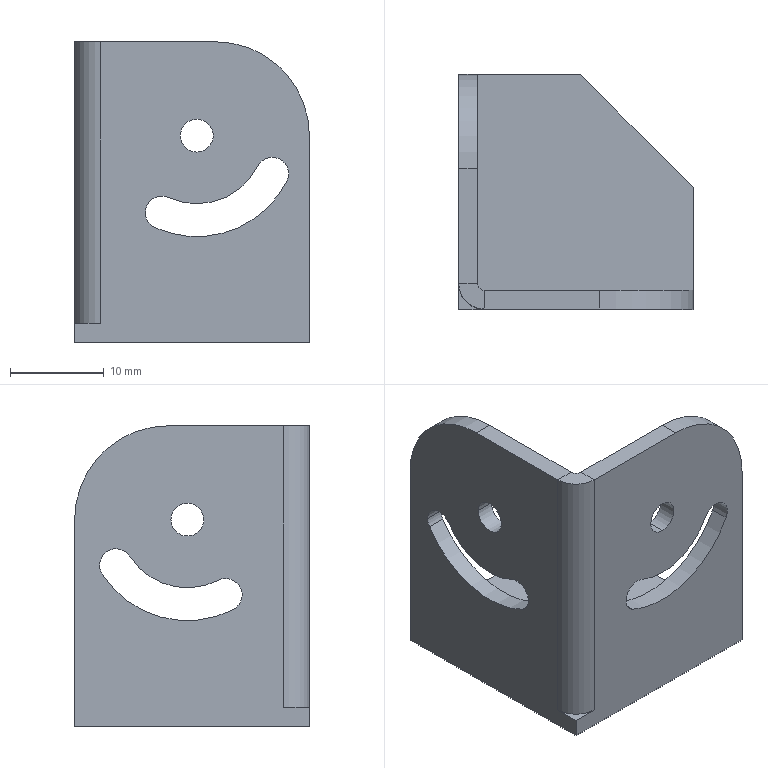Part | STEP file | 11-TG-00211 | 1 solid | 32 faces | box 25 x 25 x 32 mm | volume 3589 mm3 | cylinder 19 | plane 13 | commonest cylinder face diameters 3.5 x11 14.5 x2 20 x2 21.5 x2 1.473 x1 5.473 x1
STEP:
#1=CARTESIAN_POINT('',(19.033,-2.,17.692));
#2=VERTEX_POINT('',#1);
#3=CARTESIAN_POINT('',(20.595,-2.,15.153));
#4=VERTEX_POINT('',#3);
#5=CARTESIAN_POINT('',(19.033,-2.,15.942));
#6=DIRECTION('',(0.,1.,0.));
#7=DIRECTION('',(0.,0.,1.));
#8=AXIS2_PLACEMENT_3D('',#5,#6,#7);
#9=CIRCLE('',#8,1.75);
#10=EDGE_CURVE('',#2,#4,#9,.T.);
#11=ORIENTED_EDGE('',*,*,#10,.F.);
#12=CARTESIAN_POINT('',(19.033,0.,17.692));
#13=VERTEX_POINT('',#12);
#14=CARTESIAN_POINT('',(19.033,-10.,17.692));
#15=DIRECTION('',(0.,1.,0.));
#16=VECTOR('',#15,1000.);
#17=LINE('',#14,#16);
#18=EDGE_CURVE('',#2,#13,#17,.T.);
#19=ORIENTED_EDGE('',*,*,#18,.T.);
#20=CARTESIAN_POINT('',(20.595,0.,15.153));
#21=VERTEX_POINT('',#20);
#22=CARTESIAN_POINT('',(19.033,0.,15.942));
#23=DIRECTION('',(0.,1.,0.));
#24=DIRECTION('',(0.,0.,1.));
#25=AXIS2_PLACEMENT_3D('',#22,#23,#24);
#26=CIRCLE('',#25,1.75);
#27=EDGE_CURVE('',#13,#21,#26,.T.);
#28=ORIENTED_EDGE('',*,*,#27,.T.);
#29=CARTESIAN_POINT('',(20.595,-10.,15.153));
#30=DIRECTION('',(0.,1.,0.));
#31=VECTOR('',#30,1000.);
#32=LINE('',#29,#31);
#33=EDGE_CURVE('',#4,#21,#32,.T.);
#34=ORIENTED_EDGE('',*,*,#33,.F.);
#35=EDGE_LOOP('',(#11,#19,#28,#34));
#36=FACE_OUTER_BOUND('',#35,.T.);
#37=CARTESIAN_POINT('',(19.033,-10.,15.942));
#38=DIRECTION('',(0.,1.,0.));
#39=DIRECTION('',(0.,0.,1.));
#40=AXIS2_PLACEMENT_3D('',#37,#38,#39);
#41=CYLINDRICAL_SURFACE('',#40,1.75);
#42=ADVANCED_FACE('',(#36),#41,.F.);
#43=CARTESIAN_POINT('',(7.279,-2.,13.555));
#44=VERTEX_POINT('',#43);
#45=CARTESIAN_POINT('',(8.002,-2.,13.399));
#46=VERTEX_POINT('',#45);
#47=CARTESIAN_POINT('',(7.279,-2.,11.805));
#48=DIRECTION('',(0.,1.,0.));
#49=DIRECTION('',(0.,0.,1.));
#50=AXIS2_PLACEMENT_3D('',#47,#48,#49);
#51=CIRCLE('',#50,1.75);
#52=EDGE_CURVE('',#44,#46,#51,.T.);
#53=ORIENTED_EDGE('',*,*,#52,.F.);
#54=CARTESIAN_POINT('',(7.279,0.,13.555));
#55=VERTEX_POINT('',#54);
#56=CARTESIAN_POINT('',(7.279,-10.,13.555));
#57=DIRECTION('',(0.,1.,0.));
#58=VECTOR('',#57,1000.);
#59=LINE('',#56,#58);
#60=EDGE_CURVE('',#44,#55,#59,.T.);
#61=ORIENTED_EDGE('',*,*,#60,.T.);
#62=CARTESIAN_POINT('',(8.002,0.,13.399));
#63=VERTEX_POINT('',#62);
#64=CARTESIAN_POINT('',(7.279,0.,11.805));
#65=DIRECTION('',(0.,1.,0.));
#66=DIRECTION('',(0.,0.,1.));
#67=AXIS2_PLACEMENT_3D('',#64,#65,#66);
#68=CIRCLE('',#67,1.75);
#69=EDGE_CURVE('',#55,#63,#68,.T.);
#70=ORIENTED_EDGE('',*,*,#69,.T.);
#71=CARTESIAN_POINT('',(8.002,-10.,13.399));
#72=DIRECTION('',(0.,1.,0.));
#73=VECTOR('',#72,1000.);
#74=LINE('',#71,#73);
#75=EDGE_CURVE('',#46,#63,#74,.T.);
#76=ORIENTED_EDGE('',*,*,#75,.F.);
#77=EDGE_LOOP('',(#53,#61,#70,#76));
#78=FACE_OUTER_BOUND('',#77,.T.);
#79=CARTESIAN_POINT('',(7.279,-10.,11.805));
#80=DIRECTION('',(0.,1.,0.));
#81=DIRECTION('',(0.,0.,1.));
#82=AXIS2_PLACEMENT_3D('',#79,#80,#81);
#83=CYLINDRICAL_SURFACE('',#82,1.75);
#84=ADVANCED_FACE('',(#78),#83,.F.);
#85=CARTESIAN_POINT('',(11.,-2.,18.25));
#86=VERTEX_POINT('',#85);
#87=CARTESIAN_POINT('',(11.,-2.,21.75));
#88=VERTEX_POINT('',#87);
#89=CARTESIAN_POINT('',(11.,-2.,20.));
#90=DIRECTION('',(0.,1.,0.));
#91=DIRECTION('',(0.,0.,1.));
#92=AXIS2_PLACEMENT_3D('',#89,#90,#91);
#93=CIRCLE('',#92,1.75);
#94=EDGE_CURVE('',#86,#88,#93,.T.);
#95=ORIENTED_EDGE('',*,*,#94,.F.);
#96=CARTESIAN_POINT('',(11.,0.,18.25));
#97=VERTEX_POINT('',#96);
#98=CARTESIAN_POINT('',(11.,-10.,18.25));
#99=DIRECTION('',(0.,1.,0.));
#100=VECTOR('',#99,1000.);
#101=LINE('',#98,#100);
#102=EDGE_CURVE('',#86,#97,#101,.T.);
#103=ORIENTED_EDGE('',*,*,#102,.T.);
#104=CARTESIAN_POINT('',(11.,0.,21.75));
#105=VERTEX_POINT('',#104);
#106=CARTESIAN_POINT('',(11.,0.,20.));
#107=DIRECTION('',(0.,1.,0.));
#108=DIRECTION('',(0.,0.,1.));
#109=AXIS2_PLACEMENT_3D('',#106,#107,#108);
#110=CIRCLE('',#109,1.75);
#111=EDGE_CURVE('',#97,#105,#110,.T.);
#112=ORIENTED_EDGE('',*,*,#111,.T.);
#113=CARTESIAN_POINT('',(11.,-10.,21.75));
#114=DIRECTION('',(0.,1.,0.));
#115=VECTOR('',#114,1000.);
#116=LINE('',#113,#115);
#117=EDGE_CURVE('',#88,#105,#116,.T.);
#118=ORIENTED_EDGE('',*,*,#117,.F.);
#119=EDGE_LOOP('',(#95,#103,#112,#118));
#120=FACE_OUTER_BOUND('',#119,.T.);
#121=CARTESIAN_POINT('',(11.,-10.,20.));
#122=DIRECTION('',(0.,1.,0.));
#123=DIRECTION('',(0.,0.,1.));
#124=AXIS2_PLACEMENT_3D('',#121,#122,#123);
#125=CYLINDRICAL_SURFACE('',#124,1.75);
#126=ADVANCED_FACE('',(#120),#125,.F.);
#127=CARTESIAN_POINT('',(-2.,20.331,15.15));
#128=VERTEX_POINT('',#127);
#129=CARTESIAN_POINT('',(-2.,17.107,16.093));
#130=VERTEX_POINT('',#129);
#131=CARTESIAN_POINT('',(-2.,18.581,15.15));
#132=DIRECTION('',(1.,0.,0.));
#133=DIRECTION('',(0.,1.,0.));
#134=AXIS2_PLACEMENT_3D('',#131,#132,#133);
#135=CIRCLE('',#134,1.75);
#136=EDGE_CURVE('',#128,#130,#135,.T.);
#137=ORIENTED_EDGE('',*,*,#136,.F.);
#138=CARTESIAN_POINT('',(0.,20.331,15.15));
#139=VERTEX_POINT('',#138);
#140=CARTESIAN_POINT('',(-10.,20.331,15.15));
#141=DIRECTION('',(1.,0.,0.));
#142=VECTOR('',#141,1000.);
#143=LINE('',#140,#142);
#144=EDGE_CURVE('',#128,#139,#143,.T.);
#145=ORIENTED_EDGE('',*,*,#144,.T.);
#146=CARTESIAN_POINT('',(0.,17.107,16.093));
#147=VERTEX_POINT('',#146);
#148=CARTESIAN_POINT('',(0.,18.581,15.15));
#149=DIRECTION('',(1.,0.,0.));
#150=DIRECTION('',(0.,1.,0.));
#151=AXIS2_PLACEMENT_3D('',#148,#149,#150);
#152=CIRCLE('',#151,1.75);
#153=EDGE_CURVE('',#139,#147,#152,.T.);
#154=ORIENTED_EDGE('',*,*,#153,.T.);
#155=CARTESIAN_POINT('',(-10.,17.107,16.093));
#156=DIRECTION('',(1.,0.,0.));
#157=VECTOR('',#156,1000.);
#158=LINE('',#155,#157);
#159=EDGE_CURVE('',#130,#147,#158,.T.);
#160=ORIENTED_EDGE('',*,*,#159,.F.);
#161=EDGE_LOOP('',(#137,#145,#154,#160));
#162=FACE_OUTER_BOUND('',#161,.T.);
#163=CARTESIAN_POINT('',(-10.,18.581,15.15));
#164=DIRECTION('',(1.,0.,0.));
#165=DIRECTION('',(0.,1.,0.));
#166=AXIS2_PLACEMENT_3D('',#163,#164,#165);
#167=CYLINDRICAL_SURFACE('',#166,1.75);
#168=ADVANCED_FACE('',(#162),#167,.F.);
#169=CARTESIAN_POINT('',(-2.,9.25,20.));
#170=VERTEX_POINT('',#169);
#171=CARTESIAN_POINT('',(-2.,12.75,20.));
#172=VERTEX_POINT('',#171);
#173=CARTESIAN_POINT('',(-2.,11.,20.));
#174=DIRECTION('',(1.,0.,0.));
#175=DIRECTION('',(0.,1.,0.));
#176=AXIS2_PLACEMENT_3D('',#173,#174,#175);
#177=CIRCLE('',#176,1.75);
#178=EDGE_CURVE('',#170,#172,#177,.T.);
#179=ORIENTED_EDGE('',*,*,#178,.F.);
#180=CARTESIAN_POINT('',(0.,9.25,20.));
#181=VERTEX_POINT('',#180);
#182=CARTESIAN_POINT('',(-10.,9.25,20.));
#183=DIRECTION('',(1.,0.,0.));
#184=VECTOR('',#183,1000.);
#185=LINE('',#182,#184);
#186=EDGE_CURVE('',#170,#181,#185,.T.);
#187=ORIENTED_EDGE('',*,*,#186,.T.);
#188=CARTESIAN_POINT('',(0.,12.75,20.));
#189=VERTEX_POINT('',#188);
#190=CARTESIAN_POINT('',(0.,11.,20.));
#191=DIRECTION('',(1.,0.,0.));
#192=DIRECTION('',(0.,1.,0.));
#193=AXIS2_PLACEMENT_3D('',#190,#191,#192);
#194=CIRCLE('',#193,1.75);
#195=EDGE_CURVE('',#181,#189,#194,.T.);
#196=ORIENTED_EDGE('',*,*,#195,.T.);
#197=CARTESIAN_POINT('',(-10.,12.75,20.));
#198=DIRECTION('',(1.,0.,0.));
#199=VECTOR('',#198,1000.);
#200=LINE('',#197,#199);
#201=EDGE_CURVE('',#172,#189,#200,.T.);
#202=ORIENTED_EDGE('',*,*,#201,.F.);
#203=EDGE_LOOP('',(#179,#187,#196,#202));
#204=FACE_OUTER_BOUND('',#203,.T.);
#205=CARTESIAN_POINT('',(-10.,11.,20.));
#206=DIRECTION('',(1.,0.,0.));
#207=DIRECTION('',(0.,1.,0.));
#208=AXIS2_PLACEMENT_3D('',#205,#206,#207);
#209=CYLINDRICAL_SURFACE('',#208,1.75);
#210=ADVANCED_FACE('',(#204),#209,.F.);
#211=CARTESIAN_POINT('',(11.,-2.,20.));
#212=DIRECTION('',(0.,1.,0.));
#213=DIRECTION('',(0.,0.,1.));
#214=AXIS2_PLACEMENT_3D('',#211,#212,#213);
#215=CIRCLE('',#214,1.75);
#216=EDGE_CURVE('',#88,#86,#215,.T.);
#217=ORIENTED_EDGE('',*,*,#216,.T.);
#218=ORIENTED_EDGE('',*,*,#94,.T.);
#219=EDGE_LOOP('',(#217,#218));
#220=FACE_BOUND('',#219,.T.);
#221=CARTESIAN_POINT('',(23.,-2.,20.));
#222=VERTEX_POINT('',#221);
#223=CARTESIAN_POINT('',(23.,-2.,-2.));
#224=VERTEX_POINT('',#223);
#225=CARTESIAN_POINT('',(23.,-2.,30.));
#226=DIRECTION('',(0.,0.,-1.));
#227=VECTOR('',#226,1000.);
#228=LINE('',#225,#227);
#229=EDGE_CURVE('',#222,#224,#228,.T.);
#230=ORIENTED_EDGE('',*,*,#229,.F.);
#231=CARTESIAN_POINT('',(13.,-2.,30.));
#232=VERTEX_POINT('',#231);
#233=CARTESIAN_POINT('',(13.,-2.,20.));
#234=DIRECTION('',(0.,-1.,0.));
#235=DIRECTION('',(0.,0.,1.));
#236=AXIS2_PLACEMENT_3D('',#233,#234,#235);
#237=CIRCLE('',#236,10.);
#238=EDGE_CURVE('',#222,#232,#237,.T.);
#239=ORIENTED_EDGE('',*,*,#238,.T.);
#240=CARTESIAN_POINT('',(0.7366,-2.,30.));
#241=VERTEX_POINT('',#240);
#242=CARTESIAN_POINT('',(0.,-2.,30.));
#243=DIRECTION('',(1.,0.,0.));
#244=VECTOR('',#243,1000.);
#245=LINE('',#242,#244);
#246=EDGE_CURVE('',#241,#232,#245,.T.);
#247=ORIENTED_EDGE('',*,*,#246,.F.);
#248=CARTESIAN_POINT('',(0.7366,-2.,0.));
#249=VERTEX_POINT('',#248);
#250=CARTESIAN_POINT('',(0.7366,-2.,30.));
#251=DIRECTION('',(0.,0.,-1.));
#252=VECTOR('',#251,1000.);
#253=LINE('',#250,#252);
#254=EDGE_CURVE('',#241,#249,#253,.T.);
#255=ORIENTED_EDGE('',*,*,#254,.T.);
#256=CARTESIAN_POINT('',(-2.,-2.,0.));
#257=VERTEX_POINT('',#256);
#258=CARTESIAN_POINT('',(23.,-2.,0.));
#259=DIRECTION('',(-1.,0.,0.));
#260=VECTOR('',#259,1000.);
#261=LINE('',#258,#260);
#262=EDGE_CURVE('',#249,#257,#261,.T.);
#263=ORIENTED_EDGE('',*,*,#262,.T.);
#264=CARTESIAN_POINT('',(-2.,-2.,-2.));
#265=VERTEX_POINT('',#264);
#266=CARTESIAN_POINT('',(-2.,-2.,-2.));
#267=DIRECTION('',(0.,0.,1.));
#268=VECTOR('',#267,1000.);
#269=LINE('',#266,#268);
#270=EDGE_CURVE('',#265,#257,#269,.T.);
#271=ORIENTED_EDGE('',*,*,#270,.F.);
#272=CARTESIAN_POINT('',(23.,-2.,-2.));
#273=DIRECTION('',(-1.,0.,0.));
#274=VECTOR('',#273,1000.);
#275=LINE('',#272,#274);
#276=EDGE_CURVE('',#224,#265,#275,.T.);
#277=ORIENTED_EDGE('',*,*,#276,.F.);
#278=EDGE_LOOP('',(#230,#239,#247,#255,#263,#271,#277));
#279=FACE_OUTER_BOUND('',#278,.T.);
#280=CARTESIAN_POINT('',(6.555,-2.,10.212));
#281=VERTEX_POINT('',#280);
#282=CARTESIAN_POINT('',(11.,-2.,20.));
#283=DIRECTION('',(0.,1.,0.));
#284=DIRECTION('',(0.,0.,1.));
#285=AXIS2_PLACEMENT_3D('',#282,#283,#284);
#286=CIRCLE('',#285,10.75);
#287=EDGE_CURVE('',#4,#281,#286,.T.);
#288=ORIENTED_EDGE('',*,*,#287,.T.);
#289=CARTESIAN_POINT('',(7.279,-2.,11.805));
#290=DIRECTION('',(0.,1.,0.));
#291=DIRECTION('',(0.,0.,1.));
#292=AXIS2_PLACEMENT_3D('',#289,#290,#291);
#293=CIRCLE('',#292,1.75);
#294=EDGE_CURVE('',#281,#44,#293,.T.);
#295=ORIENTED_EDGE('',*,*,#294,.T.);
#296=ORIENTED_EDGE('',*,*,#52,.T.);
#297=CARTESIAN_POINT('',(17.471,-2.,16.731));
#298=VERTEX_POINT('',#297);
#299=CARTESIAN_POINT('',(11.,-2.,20.));
#300=DIRECTION('',(0.,-1.,0.));
#301=DIRECTION('',(0.,0.,1.));
#302=AXIS2_PLACEMENT_3D('',#299,#300,#301);
#303=CIRCLE('',#302,7.25);
#304=EDGE_CURVE('',#46,#298,#303,.T.);
#305=ORIENTED_EDGE('',*,*,#304,.T.);
#306=CARTESIAN_POINT('',(19.033,-2.,15.942));
#307=DIRECTION('',(0.,1.,0.));
#308=DIRECTION('',(0.,0.,1.));
#309=AXIS2_PLACEMENT_3D('',#306,#307,#308);
#310=CIRCLE('',#309,1.75);
#311=EDGE_CURVE('',#298,#2,#310,.T.);
#312=ORIENTED_EDGE('',*,*,#311,.T.);
#313=ORIENTED_EDGE('',*,*,#10,.T.);
#314=EDGE_LOOP('',(#288,#295,#296,#305,#312,#313));
#315=FACE_BOUND('',#314,.T.);
#316=CARTESIAN_POINT('',(0.,-2.,30.));
#317=DIRECTION('',(0.,1.,0.));
#318=DIRECTION('',(0.,0.,1.));
#319=AXIS2_PLACEMENT_3D('',#316,#317,#318);
#320=PLANE('',#319);
#321=ADVANCED_FACE('',(#220,#279,#315),#320,.F.);
#322=CARTESIAN_POINT('',(0.7366,0.,30.));
#323=VERTEX_POINT('',#322);
#324=CARTESIAN_POINT('',(13.,0.,30.));
#325=VERTEX_POINT('',#324);
#326=CARTESIAN_POINT('',(0.,0.,30.));
#327=DIRECTION('',(1.,0.,0.));
#328=VECTOR('',#327,1000.);
#329=LINE('',#326,#328);
#330=EDGE_CURVE('',#323,#325,#329,.T.);
#331=ORIENTED_EDGE('',*,*,#330,.T.);
#332=CARTESIAN_POINT('',(23.,0.,20.));
#333=VERTEX_POINT('',#332);
#334=CARTESIAN_POINT('',(13.,0.,20.));
#335=DIRECTION('',(0.,1.,0.));
#336=DIRECTION('',(0.,0.,1.));
#337=AXIS2_PLACEMENT_3D('',#334,#335,#336);
#338=CIRCLE('',#337,10.);
#339=EDGE_CURVE('',#325,#333,#338,.T.);
#340=ORIENTED_EDGE('',*,*,#339,.T.);
#341=CARTESIAN_POINT('',(23.,0.,0.));
#342=VERTEX_POINT('',#341);
#343=CARTESIAN_POINT('',(23.,0.,30.));
#344=DIRECTION('',(0.,0.,-1.));
#345=VECTOR('',#344,1000.);
#346=LINE('',#343,#345);
#347=EDGE_CURVE('',#333,#342,#346,.T.);
#348=ORIENTED_EDGE('',*,*,#347,.T.);
#349=CARTESIAN_POINT('',(0.7366,0.,0.));
#350=VERTEX_POINT('',#349);
#351=CARTESIAN_POINT('',(0.,0.,0.));
#352=DIRECTION('',(1.,0.,0.));
#353=VECTOR('',#352,1000.);
#354=LINE('',#351,#353);
#355=EDGE_CURVE('',#350,#342,#354,.T.);
#356=ORIENTED_EDGE('',*,*,#355,.F.);
#357=CARTESIAN_POINT('',(0.7366,0.,30.));
#358=DIRECTION('',(0.,0.,-1.));
#359=VECTOR('',#358,1000.);
#360=LINE('',#357,#359);
#361=EDGE_CURVE('',#323,#350,#360,.T.);
#362=ORIENTED_EDGE('',*,*,#361,.F.);
#363=EDGE_LOOP('',(#331,#340,#348,#356,#362));
#364=FACE_OUTER_BOUND('',#363,.T.);
#365=CARTESIAN_POINT('',(11.,0.,20.));
#366=DIRECTION('',(0.,1.,0.));
#367=DIRECTION('',(0.,0.,1.));
#368=AXIS2_PLACEMENT_3D('',#365,#366,#367);
#369=CIRCLE('',#368,1.75);
#370=EDGE_CURVE('',#105,#97,#369,.T.);
#371=ORIENTED_EDGE('',*,*,#370,.F.);
#372=ORIENTED_EDGE('',*,*,#111,.F.);
#373=EDGE_LOOP('',(#371,#372));
#374=FACE_BOUND('',#373,.T.);
#375=CARTESIAN_POINT('',(6.555,0.,10.212));
#376=VERTEX_POINT('',#375);
#377=CARTESIAN_POINT('',(7.279,0.,11.805));
#378=DIRECTION('',(0.,1.,0.));
#379=DIRECTION('',(0.,0.,1.));
#380=AXIS2_PLACEMENT_3D('',#377,#378,#379);
#381=CIRCLE('',#380,1.75);
#382=EDGE_CURVE('',#376,#55,#381,.T.);
#383=ORIENTED_EDGE('',*,*,#382,.F.);
#384=CARTESIAN_POINT('',(11.,0.,20.));
#385=DIRECTION('',(0.,1.,0.));
#386=DIRECTION('',(0.,0.,1.));
#387=AXIS2_PLACEMENT_3D('',#384,#385,#386);
#388=CIRCLE('',#387,10.75);
#389=EDGE_CURVE('',#21,#376,#388,.T.);
#390=ORIENTED_EDGE('',*,*,#389,.F.);
#391=ORIENTED_EDGE('',*,*,#27,.F.);
#392=CARTESIAN_POINT('',(17.471,0.,16.731));
#393=VERTEX_POINT('',#392);
#394=CARTESIAN_POINT('',(19.033,0.,15.942));
#395=DIRECTION('',(0.,1.,0.));
#396=DIRECTION('',(0.,0.,1.));
#397=AXIS2_PLACEMENT_3D('',#394,#395,#396);
#398=CIRCLE('',#397,1.75);
#399=EDGE_CURVE('',#393,#13,#398,.T.);
#400=ORIENTED_EDGE('',*,*,#399,.F.);
#401=CARTESIAN_POINT('',(11.,0.,20.));
#402=DIRECTION('',(0.,-1.,0.));
#403=DIRECTION('',(0.,0.,1.));
#404=AXIS2_PLACEMENT_3D('',#401,#402,#403);
#405=CIRCLE('',#404,7.25);
#406=EDGE_CURVE('',#63,#393,#405,.T.);
#407=ORIENTED_EDGE('',*,*,#406,.F.);
#408=ORIENTED_EDGE('',*,*,#69,.F.);
#409=EDGE_LOOP('',(#383,#390,#391,#400,#407,#408));
#410=FACE_BOUND('',#409,.T.);
#411=CARTESIAN_POINT('',(0.,0.,30.));
#412=DIRECTION('',(0.,1.,0.));
#413=DIRECTION('',(0.,0.,1.));
#414=AXIS2_PLACEMENT_3D('',#411,#412,#413);
#415=PLANE('',#414);
#416=ADVANCED_FACE('',(#364,#374,#410),#415,.T.);
#417=CARTESIAN_POINT('',(0.,23.,20.));
#418=VERTEX_POINT('',#417);
#419=CARTESIAN_POINT('',(0.,23.,0.));
#420=VERTEX_POINT('',#419);
#421=CARTESIAN_POINT('',(0.,23.,30.));
#422=DIRECTION('',(0.,0.,-1.));
#423=VECTOR('',#422,1000.);
#424=LINE('',#421,#423);
#425=EDGE_CURVE('',#418,#420,#424,.T.);
#426=ORIENTED_EDGE('',*,*,#425,.F.);
#427=CARTESIAN_POINT('',(0.,13.,30.));
#428=VERTEX_POINT('',#427);
#429=CARTESIAN_POINT('',(0.,13.,20.));
#430=DIRECTION('',(1.,0.,0.));
#431=DIRECTION('',(0.,1.,0.));
#432=AXIS2_PLACEMENT_3D('',#429,#430,#431);
#433=CIRCLE('',#432,10.);
#434=EDGE_CURVE('',#418,#428,#433,.T.);
#435=ORIENTED_EDGE('',*,*,#434,.T.);
#436=CARTESIAN_POINT('',(0.,0.7366,30.));
#437=VERTEX_POINT('',#436);
#438=CARTESIAN_POINT('',(0.,23.,30.));
#439=DIRECTION('',(0.,-1.,0.));
#440=VECTOR('',#439,1000.);
#441=LINE('',#438,#440);
#442=EDGE_CURVE('',#428,#437,#441,.T.);
#443=ORIENTED_EDGE('',*,*,#442,.T.);
#444=CARTESIAN_POINT('',(0.,0.7366,0.));
#445=VERTEX_POINT('',#444);
#446=CARTESIAN_POINT('',(0.,0.7366,30.));
#447=DIRECTION('',(0.,0.,-1.));
#448=VECTOR('',#447,1000.);
#449=LINE('',#446,#448);
#450=EDGE_CURVE('',#437,#445,#449,.T.);
#451=ORIENTED_EDGE('',*,*,#450,.T.);
#452=CARTESIAN_POINT('',(0.,23.,0.));
#453=DIRECTION('',(0.,-1.,0.));
#454=VECTOR('',#453,1000.);
#455=LINE('',#452,#454);
#456=EDGE_CURVE('',#420,#445,#455,.T.);
#457=ORIENTED_EDGE('',*,*,#456,.F.);
#458=EDGE_LOOP('',(#426,#435,#443,#451,#457));
#459=FACE_OUTER_BOUND('',#458,.T.);
#460=CARTESIAN_POINT('',(0.,11.,20.));
#461=DIRECTION('',(1.,0.,0.));
#462=DIRECTION('',(0.,1.,0.));
#463=AXIS2_PLACEMENT_3D('',#460,#461,#462);
#464=CIRCLE('',#463,1.75);
#465=EDGE_CURVE('',#189,#181,#464,.T.);
#466=ORIENTED_EDGE('',*,*,#465,.F.);
#467=ORIENTED_EDGE('',*,*,#195,.F.);
#468=EDGE_LOOP('',(#466,#467));
#469=FACE_BOUND('',#468,.T.);
#470=CARTESIAN_POINT('',(0.,20.056,14.207));
#471=VERTEX_POINT('',#470);
#472=CARTESIAN_POINT('',(0.,18.581,15.15));
#473=DIRECTION('',(1.,0.,0.));
#474=DIRECTION('',(0.,1.,0.));
#475=AXIS2_PLACEMENT_3D('',#472,#473,#474);
#476=CIRCLE('',#475,1.75);
#477=EDGE_CURVE('',#471,#139,#476,.T.);
#478=ORIENTED_EDGE('',*,*,#477,.F.);
#479=CARTESIAN_POINT('',(0.,6.117,10.423));
#480=VERTEX_POINT('',#479);
#481=CARTESIAN_POINT('',(0.,11.,20.));
#482=DIRECTION('',(1.,0.,0.));
#483=DIRECTION('',(0.,1.,0.));
#484=AXIS2_PLACEMENT_3D('',#481,#482,#483);
#485=CIRCLE('',#484,10.75);
#486=EDGE_CURVE('',#480,#471,#485,.T.);
#487=ORIENTED_EDGE('',*,*,#486,.F.);
#488=CARTESIAN_POINT('',(0.,7.707,13.541));
#489=VERTEX_POINT('',#488);
#490=CARTESIAN_POINT('',(0.,6.912,11.982));
#491=DIRECTION('',(1.,0.,0.));
#492=DIRECTION('',(0.,1.,0.));
#493=AXIS2_PLACEMENT_3D('',#490,#491,#492);
#494=CIRCLE('',#493,1.75);
#495=EDGE_CURVE('',#489,#480,#494,.T.);
#496=ORIENTED_EDGE('',*,*,#495,.F.);
#497=CARTESIAN_POINT('',(0.,11.,20.));
#498=DIRECTION('',(-1.,0.,0.));
#499=DIRECTION('',(0.,1.,0.));
#500=AXIS2_PLACEMENT_3D('',#497,#498,#499);
#501=CIRCLE('',#500,7.25);
#502=EDGE_CURVE('',#147,#489,#501,.T.);
#503=ORIENTED_EDGE('',*,*,#502,.F.);
#504=ORIENTED_EDGE('',*,*,#153,.F.);
#505=EDGE_LOOP('',(#478,#487,#496,#503,#504));
#506=FACE_BOUND('',#505,.T.);
#507=CARTESIAN_POINT('',(0.,23.,30.));
#508=DIRECTION('',(1.,0.,0.));
#509=DIRECTION('',(0.,1.,0.));
#510=AXIS2_PLACEMENT_3D('',#507,#508,#509);
#511=PLANE('',#510);
#512=ADVANCED_FACE('',(#459,#469,#506),#511,.T.);
#513=CARTESIAN_POINT('',(-2.,11.,20.));
#514=DIRECTION('',(1.,0.,0.));
#515=DIRECTION('',(0.,1.,0.));
#516=AXIS2_PLACEMENT_3D('',#513,#514,#515);
#517=CIRCLE('',#516,1.75);
#518=EDGE_CURVE('',#172,#170,#517,.T.);
#519=ORIENTED_EDGE('',*,*,#518,.T.);
#520=ORIENTED_EDGE('',*,*,#178,.T.);
#521=EDGE_LOOP('',(#519,#520));
#522=FACE_BOUND('',#521,.T.);
#523=CARTESIAN_POINT('',(-2.,13.,30.));
#524=VERTEX_POINT('',#523);
#525=CARTESIAN_POINT('',(-2.,0.7366,30.));
#526=VERTEX_POINT('',#525);
#527=CARTESIAN_POINT('',(-2.,23.,30.));
#528=DIRECTION('',(0.,-1.,0.));
#529=VECTOR('',#528,1000.);
#530=LINE('',#527,#529);
#531=EDGE_CURVE('',#524,#526,#530,.T.);
#532=ORIENTED_EDGE('',*,*,#531,.F.);
#533=CARTESIAN_POINT('',(-2.,23.,20.));
#534=VERTEX_POINT('',#533);
#535=CARTESIAN_POINT('',(-2.,13.,20.));
#536=DIRECTION('',(-1.,0.,0.));
#537=DIRECTION('',(0.,1.,0.));
#538=AXIS2_PLACEMENT_3D('',#535,#536,#537);
#539=CIRCLE('',#538,10.);
#540=EDGE_CURVE('',#524,#534,#539,.T.);
#541=ORIENTED_EDGE('',*,*,#540,.T.);
#542=CARTESIAN_POINT('',(-2.,23.,-2.));
#543=VERTEX_POINT('',#542);
#544=CARTESIAN_POINT('',(-2.,23.,30.));
#545=DIRECTION('',(0.,0.,-1.));
#546=VECTOR('',#545,1000.);
#547=LINE('',#544,#546);
#548=EDGE_CURVE('',#534,#543,#547,.T.);
#549=ORIENTED_EDGE('',*,*,#548,.T.);
#550=CARTESIAN_POINT('',(-2.,-2.,-2.));
#551=DIRECTION('',(0.,1.,0.));
#552=VECTOR('',#551,1000.);
#553=LINE('',#550,#552);
#554=EDGE_CURVE('',#265,#543,#553,.T.);
#555=ORIENTED_EDGE('',*,*,#554,.F.);
#556=ORIENTED_EDGE('',*,*,#270,.T.);
#557=CARTESIAN_POINT('',(-2.,0.7366,0.));
#558=VERTEX_POINT('',#557);
#559=CARTESIAN_POINT('',(-2.,-2.,0.));
#560=DIRECTION('',(0.,1.,0.));
#561=VECTOR('',#560,1000.);
#562=LINE('',#559,#561);
#563=EDGE_CURVE('',#257,#558,#562,.T.);
#564=ORIENTED_EDGE('',*,*,#563,.T.);
#565=CARTESIAN_POINT('',(-2.,0.7366,30.));
#566=DIRECTION('',(0.,0.,-1.));
#567=VECTOR('',#566,1000.);
#568=LINE('',#565,#567);
#569=EDGE_CURVE('',#526,#558,#568,.T.);
#570=ORIENTED_EDGE('',*,*,#569,.F.);
#571=EDGE_LOOP('',(#532,#541,#549,#555,#556,#564,#570));
#572=FACE_OUTER_BOUND('',#571,.T.);
#573=CARTESIAN_POINT('',(-2.,6.117,10.423));
#574=VERTEX_POINT('',#573);
#575=CARTESIAN_POINT('',(-2.,20.056,14.207));
#576=VERTEX_POINT('',#575);
#577=CARTESIAN_POINT('',(-2.,11.,20.));
#578=DIRECTION('',(1.,0.,0.));
#579=DIRECTION('',(0.,1.,0.));
#580=AXIS2_PLACEMENT_3D('',#577,#578,#579);
#581=CIRCLE('',#580,10.75);
#582=EDGE_CURVE('',#574,#576,#581,.T.);
#583=ORIENTED_EDGE('',*,*,#582,.T.);
#584=CARTESIAN_POINT('',(-2.,18.581,15.15));
#585=DIRECTION('',(1.,0.,0.));
#586=DIRECTION('',(0.,1.,0.));
#587=AXIS2_PLACEMENT_3D('',#584,#585,#586);
#588=CIRCLE('',#587,1.75);
#589=EDGE_CURVE('',#576,#128,#588,.T.);
#590=ORIENTED_EDGE('',*,*,#589,.T.);
#591=ORIENTED_EDGE('',*,*,#136,.T.);
#592=CARTESIAN_POINT('',(-2.,7.707,13.541));
#593=VERTEX_POINT('',#592);
#594=CARTESIAN_POINT('',(-2.,11.,20.));
#595=DIRECTION('',(-1.,0.,0.));
#596=DIRECTION('',(0.,1.,0.));
#597=AXIS2_PLACEMENT_3D('',#594,#595,#596);
#598=CIRCLE('',#597,7.25);
#599=EDGE_CURVE('',#130,#593,#598,.T.);
#600=ORIENTED_EDGE('',*,*,#599,.T.);
#601=CARTESIAN_POINT('',(-2.,6.912,11.982));
#602=DIRECTION('',(1.,0.,0.));
#603=DIRECTION('',(0.,1.,0.));
#604=AXIS2_PLACEMENT_3D('',#601,#602,#603);
#605=CIRCLE('',#604,1.75);
#606=EDGE_CURVE('',#593,#574,#605,.T.);
#607=ORIENTED_EDGE('',*,*,#606,.T.);
#608=EDGE_LOOP('',(#583,#590,#591,#600,#607));
#609=FACE_BOUND('',#608,.T.);
#610=CARTESIAN_POINT('',(-2.,23.,30.));
#611=DIRECTION('',(1.,0.,0.));
#612=DIRECTION('',(0.,1.,0.));
#613=AXIS2_PLACEMENT_3D('',#610,#611,#612);
#614=PLANE('',#613);
#615=ADVANCED_FACE('',(#522,#572,#609),#614,.F.);
#616=CARTESIAN_POINT('',(0.7366,0.,30.));
#617=DIRECTION('',(0.,-1.,0.));
#618=VECTOR('',#617,1000.);
#619=LINE('',#616,#618);
#620=EDGE_CURVE('',#323,#241,#619,.T.);
#621=ORIENTED_EDGE('',*,*,#620,.F.);
#622=CARTESIAN_POINT('',(0.7366,0.7366,30.));
#623=DIRECTION('',(0.,0.,1.));
#624=DIRECTION('',(-1.,0.,0.));
#625=AXIS2_PLACEMENT_3D('',#622,#623,#624);
#626=CIRCLE('',#625,0.7366);
#627=EDGE_CURVE('',#437,#323,#626,.T.);
#628=ORIENTED_EDGE('',*,*,#627,.F.);
#629=CARTESIAN_POINT('',(-2.,0.7366,30.));
#630=DIRECTION('',(1.,0.,0.));
#631=VECTOR('',#630,1000.);
#632=LINE('',#629,#631);
#633=EDGE_CURVE('',#526,#437,#632,.T.);
#634=ORIENTED_EDGE('',*,*,#633,.F.);
#635=CARTESIAN_POINT('',(0.7366,0.7366,30.));
#636=DIRECTION('',(0.,0.,1.));
#637=DIRECTION('',(1.,0.,0.));
#638=AXIS2_PLACEMENT_3D('',#635,#636,#637);
#639=CIRCLE('',#638,2.737);
#640=EDGE_CURVE('',#526,#241,#639,.T.);
#641=ORIENTED_EDGE('',*,*,#640,.T.);
#642=EDGE_LOOP('',(#621,#628,#634,#641));
#643=FACE_OUTER_BOUND('',#642,.T.);
#644=CARTESIAN_POINT('',(0.7366,0.,30.));
#645=DIRECTION('',(0.,0.,1.));
#646=DIRECTION('',(1.,0.,0.));
#647=AXIS2_PLACEMENT_3D('',#644,#645,#646);
#648=PLANE('',#647);
#649=ADVANCED_FACE('',(#643),#648,.T.);
#650=ORIENTED_EDGE('',*,*,#246,.T.);
#651=CARTESIAN_POINT('',(13.,0.7366,30.));
#652=DIRECTION('',(0.,1.,0.));
#653=VECTOR('',#652,1000.);
#654=LINE('',#651,#653);
#655=EDGE_CURVE('',#232,#325,#654,.T.);
#656=ORIENTED_EDGE('',*,*,#655,.T.);
#657=ORIENTED_EDGE('',*,*,#330,.F.);
#658=ORIENTED_EDGE('',*,*,#620,.T.);
#659=EDGE_LOOP('',(#650,#656,#657,#658));
#660=FACE_OUTER_BOUND('',#659,.T.);
#661=CARTESIAN_POINT('',(-2.,0.7366,30.));
#662=DIRECTION('',(0.,0.,1.));
#663=DIRECTION('',(1.,0.,0.));
#664=AXIS2_PLACEMENT_3D('',#661,#662,#663);
#665=PLANE('',#664);
#666=ADVANCED_FACE('',(#660),#665,.T.);
#667=CARTESIAN_POINT('',(23.,11.,-2.));
#668=VERTEX_POINT('',#667);
#669=CARTESIAN_POINT('',(23.,-2.,-2.));
#670=DIRECTION('',(0.,-1.,0.));
#671=VECTOR('',#670,1000.);
#672=LINE('',#669,#671);
#673=EDGE_CURVE('',#668,#224,#672,.T.);
#674=ORIENTED_EDGE('',*,*,#673,.F.);
#675=CARTESIAN_POINT('',(23.,11.,0.));
#676=VERTEX_POINT('',#675);
#677=CARTESIAN_POINT('',(23.,11.,30.));
#678=DIRECTION('',(0.,0.,1.));
#679=VECTOR('',#678,1000.);
#680=LINE('',#677,#679);
#681=EDGE_CURVE('',#668,#676,#680,.T.);
#682=ORIENTED_EDGE('',*,*,#681,.T.);
#683=CARTESIAN_POINT('',(23.,-2.,0.));
#684=DIRECTION('',(0.,-1.,0.));
#685=VECTOR('',#684,1000.);
#686=LINE('',#683,#685);
#687=EDGE_CURVE('',#676,#342,#686,.T.);
#688=ORIENTED_EDGE('',*,*,#687,.T.);
#689=ORIENTED_EDGE('',*,*,#347,.F.);
#690=CARTESIAN_POINT('',(23.,0.,20.));
#691=DIRECTION('',(0.,-1.,0.));
#692=VECTOR('',#691,1000.);
#693=LINE('',#690,#692);
#694=EDGE_CURVE('',#333,#222,#693,.T.);
#695=ORIENTED_EDGE('',*,*,#694,.T.);
#696=ORIENTED_EDGE('',*,*,#229,.T.);
#697=EDGE_LOOP('',(#674,#682,#688,#689,#695,#696));
#698=FACE_OUTER_BOUND('',#697,.T.);
#699=CARTESIAN_POINT('',(23.,0.,30.));
#700=DIRECTION('',(1.,0.,0.));
#701=DIRECTION('',(0.,0.,-1.));
#702=AXIS2_PLACEMENT_3D('',#699,#700,#701);
#703=PLANE('',#702);
#704=ADVANCED_FACE('',(#698),#703,.T.);
#705=CARTESIAN_POINT('',(0.7366,0.7366,0.));
#706=DIRECTION('',(0.,0.,1.));
#707=DIRECTION('',(-1.,0.,0.));
#708=AXIS2_PLACEMENT_3D('',#705,#706,#707);
#709=CIRCLE('',#708,0.7366);
#710=EDGE_CURVE('',#445,#350,#709,.T.);
#711=ORIENTED_EDGE('',*,*,#710,.F.);
#712=ORIENTED_EDGE('',*,*,#450,.F.);
#713=ORIENTED_EDGE('',*,*,#627,.T.);
#714=ORIENTED_EDGE('',*,*,#361,.T.);
#715=EDGE_LOOP('',(#711,#712,#713,#714));
#716=FACE_OUTER_BOUND('',#715,.T.);
#717=CARTESIAN_POINT('',(0.7366,0.7366,30.));
#718=DIRECTION('',(0.,0.,-1.));
#719=DIRECTION('',(-1.,0.,0.));
#720=AXIS2_PLACEMENT_3D('',#717,#718,#719);
#721=CYLINDRICAL_SURFACE('',#720,0.7366);
#722=ADVANCED_FACE('',(#716),#721,.F.);
#723=CARTESIAN_POINT('',(11.,23.,0.));
#724=VERTEX_POINT('',#723);
#725=CARTESIAN_POINT('',(23.,23.,0.));
#726=DIRECTION('',(1.,0.,0.));
#727=VECTOR('',#726,1000.);
#728=LINE('',#725,#727);
#729=EDGE_CURVE('',#420,#724,#728,.T.);
#730=ORIENTED_EDGE('',*,*,#729,.T.);
#731=CARTESIAN_POINT('',(11.,23.,-2.));
#732=VERTEX_POINT('',#731);
#733=CARTESIAN_POINT('',(11.,23.,30.));
#734=DIRECTION('',(0.,0.,-1.));
#735=VECTOR('',#734,1000.);
#736=LINE('',#733,#735);
#737=EDGE_CURVE('',#724,#732,#736,.T.);
#738=ORIENTED_EDGE('',*,*,#737,.T.);
#739=CARTESIAN_POINT('',(23.,23.,-2.));
#740=DIRECTION('',(1.,0.,0.));
#741=VECTOR('',#740,1000.);
#742=LINE('',#739,#741);
#743=EDGE_CURVE('',#543,#732,#742,.T.);
#744=ORIENTED_EDGE('',*,*,#743,.F.);
#745=ORIENTED_EDGE('',*,*,#548,.F.);
#746=CARTESIAN_POINT('',(0.,23.,20.));
#747=DIRECTION('',(1.,0.,0.));
#748=VECTOR('',#747,1000.);
#749=LINE('',#746,#748);
#750=EDGE_CURVE('',#534,#418,#749,.T.);
#751=ORIENTED_EDGE('',*,*,#750,.T.);
#752=ORIENTED_EDGE('',*,*,#425,.T.);
#753=EDGE_LOOP('',(#730,#738,#744,#745,#751,#752));
#754=FACE_OUTER_BOUND('',#753,.T.);
#755=CARTESIAN_POINT('',(-2.,23.,30.));
#756=DIRECTION('',(0.,1.,0.));
#757=DIRECTION('',(0.,0.,1.));
#758=AXIS2_PLACEMENT_3D('',#755,#756,#757);
#759=PLANE('',#758);
#760=ADVANCED_FACE('',(#754),#759,.T.);
#761=CARTESIAN_POINT('',(0.7366,0.7366,0.));
#762=DIRECTION('',(0.,0.,1.));
#763=DIRECTION('',(1.,0.,0.));
#764=AXIS2_PLACEMENT_3D('',#761,#762,#763);
#765=CIRCLE('',#764,2.737);
#766=EDGE_CURVE('',#558,#249,#765,.T.);
#767=ORIENTED_EDGE('',*,*,#766,.T.);
#768=ORIENTED_EDGE('',*,*,#254,.F.);
#769=ORIENTED_EDGE('',*,*,#640,.F.);
#770=ORIENTED_EDGE('',*,*,#569,.T.);
#771=EDGE_LOOP('',(#767,#768,#769,#770));
#772=FACE_OUTER_BOUND('',#771,.T.);
#773=CARTESIAN_POINT('',(0.7366,0.7366,30.));
#774=DIRECTION('',(0.,0.,-1.));
#775=DIRECTION('',(-1.,0.,0.));
#776=AXIS2_PLACEMENT_3D('',#773,#774,#775);
#777=CYLINDRICAL_SURFACE('',#776,2.737);
#778=ADVANCED_FACE('',(#772),#777,.T.);
#779=ORIENTED_EDGE('',*,*,#442,.F.);
#780=CARTESIAN_POINT('',(-2.,13.,30.));
#781=DIRECTION('',(-1.,0.,0.));
#782=VECTOR('',#781,1000.);
#783=LINE('',#780,#782);
#784=EDGE_CURVE('',#428,#524,#783,.T.);
#785=ORIENTED_EDGE('',*,*,#784,.T.);
#786=ORIENTED_EDGE('',*,*,#531,.T.);
#787=ORIENTED_EDGE('',*,*,#633,.T.);
#788=EDGE_LOOP('',(#779,#785,#786,#787));
#789=FACE_OUTER_BOUND('',#788,.T.);
#790=CARTESIAN_POINT('',(0.7366,0.7366,30.));
#791=DIRECTION('',(0.,0.,-1.));
#792=DIRECTION('',(-1.,0.,0.));
#793=AXIS2_PLACEMENT_3D('',#790,#791,#792);
#794=PLANE('',#793);
#795=ADVANCED_FACE('',(#789),#794,.F.);
#796=ORIENTED_EDGE('',*,*,#339,.F.);
#797=ORIENTED_EDGE('',*,*,#655,.F.);
#798=ORIENTED_EDGE('',*,*,#238,.F.);
#799=ORIENTED_EDGE('',*,*,#694,.F.);
#800=EDGE_LOOP('',(#796,#797,#798,#799));
#801=FACE_OUTER_BOUND('',#800,.T.);
#802=CARTESIAN_POINT('',(13.,0.,20.));
#803=DIRECTION('',(0.,-1.,0.));
#804=DIRECTION('',(0.,0.,-1.));
#805=AXIS2_PLACEMENT_3D('',#802,#803,#804);
#806=CYLINDRICAL_SURFACE('',#805,10.);
#807=ADVANCED_FACE('',(#801),#806,.T.);
#808=ORIENTED_EDGE('',*,*,#540,.F.);
#809=ORIENTED_EDGE('',*,*,#784,.F.);
#810=ORIENTED_EDGE('',*,*,#434,.F.);
#811=ORIENTED_EDGE('',*,*,#750,.F.);
#812=EDGE_LOOP('',(#808,#809,#810,#811));
#813=FACE_OUTER_BOUND('',#812,.T.);
#814=CARTESIAN_POINT('',(-2.,13.,20.));
#815=DIRECTION('',(-1.,0.,0.));
#816=DIRECTION('',(0.,0.,1.));
#817=AXIS2_PLACEMENT_3D('',#814,#815,#816);
#818=CYLINDRICAL_SURFACE('',#817,10.);
#819=ADVANCED_FACE('',(#813),#818,.T.);
#820=ORIENTED_EDGE('',*,*,#186,.F.);
#821=ORIENTED_EDGE('',*,*,#518,.F.);
#822=ORIENTED_EDGE('',*,*,#201,.T.);
#823=ORIENTED_EDGE('',*,*,#465,.T.);
#824=EDGE_LOOP('',(#820,#821,#822,#823));
#825=FACE_OUTER_BOUND('',#824,.T.);
#826=CARTESIAN_POINT('',(-10.,11.,20.));
#827=DIRECTION('',(1.,0.,0.));
#828=DIRECTION('',(0.,1.,0.));
#829=AXIS2_PLACEMENT_3D('',#826,#827,#828);
#830=CYLINDRICAL_SURFACE('',#829,1.75);
#831=ADVANCED_FACE('',(#825),#830,.F.);
#832=ORIENTED_EDGE('',*,*,#144,.F.);
#833=ORIENTED_EDGE('',*,*,#589,.F.);
#834=CARTESIAN_POINT('',(-10.,20.056,14.207));
#835=DIRECTION('',(1.,0.,0.));
#836=VECTOR('',#835,1000.);
#837=LINE('',#834,#836);
#838=EDGE_CURVE('',#576,#471,#837,.T.);
#839=ORIENTED_EDGE('',*,*,#838,.T.);
#840=ORIENTED_EDGE('',*,*,#477,.T.);
#841=EDGE_LOOP('',(#832,#833,#839,#840));
#842=FACE_OUTER_BOUND('',#841,.T.);
#843=CARTESIAN_POINT('',(-10.,18.581,15.15));
#844=DIRECTION('',(1.,0.,0.));
#845=DIRECTION('',(0.,1.,0.));
#846=AXIS2_PLACEMENT_3D('',#843,#844,#845);
#847=CYLINDRICAL_SURFACE('',#846,1.75);
#848=ADVANCED_FACE('',(#842),#847,.F.);
#849=CARTESIAN_POINT('',(-10.,6.117,10.423));
#850=DIRECTION('',(1.,0.,0.));
#851=VECTOR('',#850,1000.);
#852=LINE('',#849,#851);
#853=EDGE_CURVE('',#574,#480,#852,.T.);
#854=ORIENTED_EDGE('',*,*,#853,.T.);
#855=ORIENTED_EDGE('',*,*,#486,.T.);
#856=ORIENTED_EDGE('',*,*,#838,.F.);
#857=ORIENTED_EDGE('',*,*,#582,.F.);
#858=EDGE_LOOP('',(#854,#855,#856,#857));
#859=FACE_OUTER_BOUND('',#858,.T.);
#860=CARTESIAN_POINT('',(-10.,11.,20.));
#861=DIRECTION('',(1.,0.,0.));
#862=DIRECTION('',(0.,1.,0.));
#863=AXIS2_PLACEMENT_3D('',#860,#861,#862);
#864=CYLINDRICAL_SURFACE('',#863,10.75);
#865=ADVANCED_FACE('',(#859),#864,.F.);
#866=CARTESIAN_POINT('',(-10.,7.707,13.541));
#867=DIRECTION('',(1.,0.,0.));
#868=VECTOR('',#867,1000.);
#869=LINE('',#866,#868);
#870=EDGE_CURVE('',#593,#489,#869,.T.);
#871=ORIENTED_EDGE('',*,*,#870,.T.);
#872=ORIENTED_EDGE('',*,*,#495,.T.);
#873=ORIENTED_EDGE('',*,*,#853,.F.);
#874=ORIENTED_EDGE('',*,*,#606,.F.);
#875=EDGE_LOOP('',(#871,#872,#873,#874));
#876=FACE_OUTER_BOUND('',#875,.T.);
#877=CARTESIAN_POINT('',(-10.,6.912,11.982));
#878=DIRECTION('',(1.,0.,0.));
#879=DIRECTION('',(0.,1.,0.));
#880=AXIS2_PLACEMENT_3D('',#877,#878,#879);
#881=CYLINDRICAL_SURFACE('',#880,1.75);
#882=ADVANCED_FACE('',(#876),#881,.F.);
#883=ORIENTED_EDGE('',*,*,#159,.T.);
#884=ORIENTED_EDGE('',*,*,#502,.T.);
#885=ORIENTED_EDGE('',*,*,#870,.F.);
#886=ORIENTED_EDGE('',*,*,#599,.F.);
#887=EDGE_LOOP('',(#883,#884,#885,#886));
#888=FACE_OUTER_BOUND('',#887,.T.);
#889=CARTESIAN_POINT('',(-10.,11.,20.));
#890=DIRECTION('',(1.,0.,0.));
#891=DIRECTION('',(0.,1.,0.));
#892=AXIS2_PLACEMENT_3D('',#889,#890,#891);
#893=CYLINDRICAL_SURFACE('',#892,7.25);
#894=ADVANCED_FACE('',(#888),#893,.T.);
#895=ORIENTED_EDGE('',*,*,#102,.F.);
#896=ORIENTED_EDGE('',*,*,#216,.F.);
#897=ORIENTED_EDGE('',*,*,#117,.T.);
#898=ORIENTED_EDGE('',*,*,#370,.T.);
#899=EDGE_LOOP('',(#895,#896,#897,#898));
#900=FACE_OUTER_BOUND('',#899,.T.);
#901=CARTESIAN_POINT('',(11.,-10.,20.));
#902=DIRECTION('',(0.,1.,0.));
#903=DIRECTION('',(0.,0.,1.));
#904=AXIS2_PLACEMENT_3D('',#901,#902,#903);
#905=CYLINDRICAL_SURFACE('',#904,1.75);
#906=ADVANCED_FACE('',(#900),#905,.F.);
#907=ORIENTED_EDGE('',*,*,#60,.F.);
#908=ORIENTED_EDGE('',*,*,#294,.F.);
#909=CARTESIAN_POINT('',(6.555,-10.,10.212));
#910=DIRECTION('',(0.,1.,0.));
#911=VECTOR('',#910,1000.);
#912=LINE('',#909,#911);
#913=EDGE_CURVE('',#281,#376,#912,.T.);
#914=ORIENTED_EDGE('',*,*,#913,.T.);
#915=ORIENTED_EDGE('',*,*,#382,.T.);
#916=EDGE_LOOP('',(#907,#908,#914,#915));
#917=FACE_OUTER_BOUND('',#916,.T.);
#918=CARTESIAN_POINT('',(7.279,-10.,11.805));
#919=DIRECTION('',(0.,1.,0.));
#920=DIRECTION('',(0.,0.,1.));
#921=AXIS2_PLACEMENT_3D('',#918,#919,#920);
#922=CYLINDRICAL_SURFACE('',#921,1.75);
#923=ADVANCED_FACE('',(#917),#922,.F.);
#924=ORIENTED_EDGE('',*,*,#33,.T.);
#925=ORIENTED_EDGE('',*,*,#389,.T.);
#926=ORIENTED_EDGE('',*,*,#913,.F.);
#927=ORIENTED_EDGE('',*,*,#287,.F.);
#928=EDGE_LOOP('',(#924,#925,#926,#927));
#929=FACE_OUTER_BOUND('',#928,.T.);
#930=CARTESIAN_POINT('',(11.,-10.,20.));
#931=DIRECTION('',(0.,1.,0.));
#932=DIRECTION('',(0.,0.,1.));
#933=AXIS2_PLACEMENT_3D('',#930,#931,#932);
#934=CYLINDRICAL_SURFACE('',#933,10.75);
#935=ADVANCED_FACE('',(#929),#934,.F.);
#936=ORIENTED_EDGE('',*,*,#18,.F.);
#937=ORIENTED_EDGE('',*,*,#311,.F.);
#938=CARTESIAN_POINT('',(17.471,-10.,16.731));
#939=DIRECTION('',(0.,1.,0.));
#940=VECTOR('',#939,1000.);
#941=LINE('',#938,#940);
#942=EDGE_CURVE('',#298,#393,#941,.T.);
#943=ORIENTED_EDGE('',*,*,#942,.T.);
#944=ORIENTED_EDGE('',*,*,#399,.T.);
#945=EDGE_LOOP('',(#936,#937,#943,#944));
#946=FACE_OUTER_BOUND('',#945,.T.);
#947=CARTESIAN_POINT('',(19.033,-10.,15.942));
#948=DIRECTION('',(0.,1.,0.));
#949=DIRECTION('',(0.,0.,1.));
#950=AXIS2_PLACEMENT_3D('',#947,#948,#949);
#951=CYLINDRICAL_SURFACE('',#950,1.75);
#952=ADVANCED_FACE('',(#946),#951,.F.);
#953=ORIENTED_EDGE('',*,*,#75,.T.);
#954=ORIENTED_EDGE('',*,*,#406,.T.);
#955=ORIENTED_EDGE('',*,*,#942,.F.);
#956=ORIENTED_EDGE('',*,*,#304,.F.);
#957=EDGE_LOOP('',(#953,#954,#955,#956));
#958=FACE_OUTER_BOUND('',#957,.T.);
#959=CARTESIAN_POINT('',(11.,-10.,20.));
#960=DIRECTION('',(0.,1.,0.));
#961=DIRECTION('',(0.,0.,1.));
#962=AXIS2_PLACEMENT_3D('',#959,#960,#961);
#963=CYLINDRICAL_SURFACE('',#962,7.25);
#964=ADVANCED_FACE('',(#958),#963,.T.);
#965=ORIENTED_EDGE('',*,*,#687,.F.);
#966=CARTESIAN_POINT('',(17.,17.,0.));
#967=DIRECTION('',(-0.7071,0.7071,0.));
#968=VECTOR('',#967,1000.);
#969=LINE('',#966,#968);
#970=EDGE_CURVE('',#676,#724,#969,.T.);
#971=ORIENTED_EDGE('',*,*,#970,.T.);
#972=ORIENTED_EDGE('',*,*,#729,.F.);
#973=ORIENTED_EDGE('',*,*,#456,.T.);
#974=ORIENTED_EDGE('',*,*,#710,.T.);
#975=ORIENTED_EDGE('',*,*,#355,.T.);
#976=EDGE_LOOP('',(#965,#971,#972,#973,#974,#975));
#977=FACE_OUTER_BOUND('',#976,.T.);
#978=CARTESIAN_POINT('',(0.,0.,0.));
#979=DIRECTION('',(0.,0.,1.));
#980=DIRECTION('',(1.,0.,0.));
#981=AXIS2_PLACEMENT_3D('',#978,#979,#980);
#982=PLANE('',#981);
#983=ADVANCED_FACE('',(#977),#982,.T.);
#984=ORIENTED_EDGE('',*,*,#743,.T.);
#985=CARTESIAN_POINT('',(23.,11.,-2.));
#986=DIRECTION('',(0.7071,-0.7071,0.));
#987=VECTOR('',#986,1000.);
#988=LINE('',#985,#987);
#989=EDGE_CURVE('',#732,#668,#988,.T.);
#990=ORIENTED_EDGE('',*,*,#989,.T.);
#991=ORIENTED_EDGE('',*,*,#673,.T.);
#992=ORIENTED_EDGE('',*,*,#276,.T.);
#993=ORIENTED_EDGE('',*,*,#554,.T.);
#994=EDGE_LOOP('',(#984,#990,#991,#992,#993));
#995=FACE_OUTER_BOUND('',#994,.T.);
#996=CARTESIAN_POINT('',(0.,0.,-2.));
#997=DIRECTION('',(0.,0.,1.));
#998=DIRECTION('',(1.,0.,0.));
#999=AXIS2_PLACEMENT_3D('',#996,#997,#998);
#1000=PLANE('',#999);
#1001=ADVANCED_FACE('',(#995),#1000,.F.);
#1002=ORIENTED_EDGE('',*,*,#766,.F.);
#1003=ORIENTED_EDGE('',*,*,#563,.F.);
#1004=ORIENTED_EDGE('',*,*,#262,.F.);
#1005=EDGE_LOOP('',(#1002,#1003,#1004));
#1006=FACE_OUTER_BOUND('',#1005,.T.);
#1007=CARTESIAN_POINT('',(0.,0.,0.));
#1008=DIRECTION('',(0.,0.,1.));
#1009=DIRECTION('',(1.,0.,0.));
#1010=AXIS2_PLACEMENT_3D('',#1007,#1008,#1009);
#1011=PLANE('',#1010);
#1012=ADVANCED_FACE('',(#1006),#1011,.T.);
#1013=ORIENTED_EDGE('',*,*,#989,.F.);
#1014=ORIENTED_EDGE('',*,*,#737,.F.);
#1015=ORIENTED_EDGE('',*,*,#970,.F.);
#1016=ORIENTED_EDGE('',*,*,#681,.F.);
#1017=EDGE_LOOP('',(#1013,#1014,#1015,#1016));
#1018=FACE_OUTER_BOUND('',#1017,.T.);
#1019=CARTESIAN_POINT('',(23.,11.,30.));
#1020=DIRECTION('',(-0.7071,-0.7071,0.));
#1021=DIRECTION('',(0.,0.,1.));
#1022=AXIS2_PLACEMENT_3D('',#1019,#1020,#1021);
#1023=PLANE('',#1022);
#1024=ADVANCED_FACE('',(#1018),#1023,.F.);
#1025=CLOSED_SHELL('',(#42,#84,#126,#168,#210,#321,#416,#512,#615,#649,#666,#704,#722,#760,#778,#795,#807,#819,#831,#848,#865,#882,#894,#906,#923,#935,#952,#964,#983,#1001,#1012,#1024));
#1026=MANIFOLD_SOLID_BREP('',#1025);
#1027=CARTESIAN_POINT('',(0.,0.,0.));
#1028=DIRECTION('',(0.,0.,1.));
#1029=DIRECTION('',(1.,0.,0.));
#1030=AXIS2_PLACEMENT_3D('',#1027,#1028,#1029);
#1031=(LENGTH_UNIT()NAMED_UNIT(*)SI_UNIT(.MILLI.,.METRE.));
#1032=UNCERTAINTY_MEASURE_WITH_UNIT(LENGTH_MEASURE(0.00001),#1031,'','');
#1033=(NAMED_UNIT(*)PLANE_ANGLE_UNIT()SI_UNIT($,.RADIAN.));
#1034=(NAMED_UNIT(*)SI_UNIT($,.STERADIAN.)SOLID_ANGLE_UNIT());
#1035=(GEOMETRIC_REPRESENTATION_CONTEXT(3)GLOBAL_UNCERTAINTY_ASSIGNED_CONTEXT((#1032))GLOBAL_UNIT_ASSIGNED_CONTEXT((#1031,#1033,#1034))REPRESENTATION_CONTEXT('',''));
#1036=ADVANCED_BREP_SHAPE_REPRESENTATION('',(#1026,#1030),#1035);